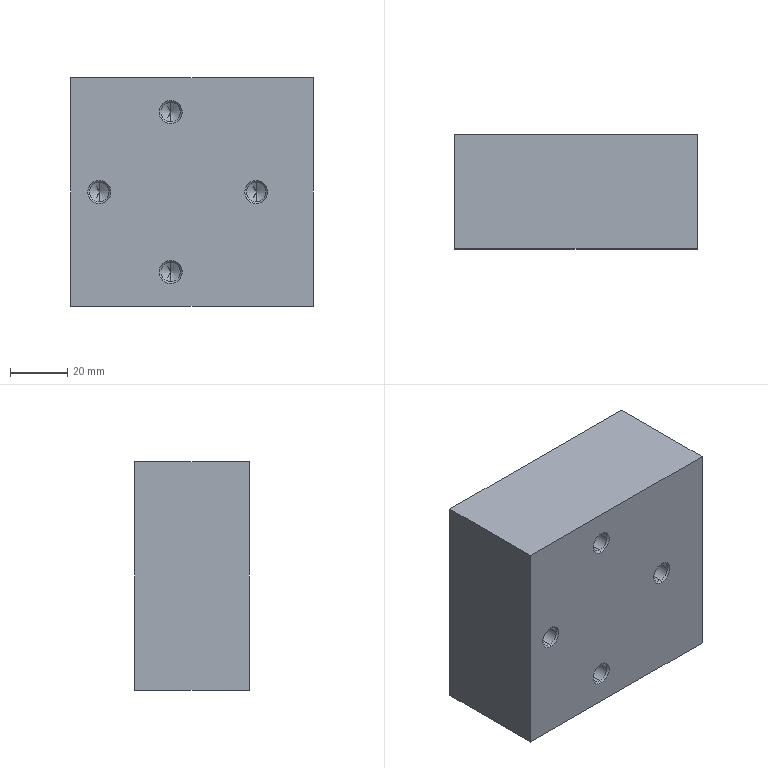Part | SolidWorks | features ICE 2, Extrusion 1, HoleWzd 1 | 1 solid | 45 faces | box 85 x 40 x 80 mm | volume 265399 mm3 | cone 16 | plane 16 | cylinder 13 | commonest cylinder face diameters 6.8 x8 2 x3 16.4 x2
STEP:
#1=CARTESIAN_POINT('',(-7.5,0.625,-24.6));
#2=VERTEX_POINT('',#1);
#3=CARTESIAN_POINT('',(-7.5,0.625,-31.4));
#4=VERTEX_POINT('',#3);
#5=CARTESIAN_POINT('',(-7.5,0.625,-28.));
#6=DIRECTION('',(0.,-1.,0.));
#7=DIRECTION('',(0.,0.,-1.));
#8=AXIS2_PLACEMENT_3D('',#5,#6,#7);
#9=CIRCLE('',#8,3.4);
#10=EDGE_CURVE('',#2,#4,#9,.T.);
#11=ORIENTED_EDGE('',*,*,#10,.F.);
#12=CARTESIAN_POINT('',(-7.5,0.,-23.975));
#13=VERTEX_POINT('',#12);
#14=CARTESIAN_POINT('',(-7.5,0.,-23.975));
#15=DIRECTION('',(0.,-0.7071,0.7071));
#16=VECTOR('',#15,1000.);
#17=LINE('',#14,#16);
#18=EDGE_CURVE('',#2,#13,#17,.T.);
#19=ORIENTED_EDGE('',*,*,#18,.T.);
#20=CARTESIAN_POINT('',(-7.5,0.,-32.025));
#21=VERTEX_POINT('',#20);
#22=CARTESIAN_POINT('',(-7.5,0.,-28.));
#23=DIRECTION('',(0.,-1.,0.));
#24=DIRECTION('',(0.,0.,-1.));
#25=AXIS2_PLACEMENT_3D('',#22,#23,#24);
#26=CIRCLE('',#25,4.025);
#27=EDGE_CURVE('',#13,#21,#26,.T.);
#28=ORIENTED_EDGE('',*,*,#27,.T.);
#29=CARTESIAN_POINT('',(-7.5,0.,-32.025));
#30=DIRECTION('',(0.,-0.7071,-0.7071));
#31=VECTOR('',#30,1000.);
#32=LINE('',#29,#31);
#33=EDGE_CURVE('',#4,#21,#32,.T.);
#34=ORIENTED_EDGE('',*,*,#33,.F.);
#35=EDGE_LOOP('',(#11,#19,#28,#34));
#36=FACE_OUTER_BOUND('',#35,.T.);
#37=CARTESIAN_POINT('',(-7.5,0.,-28.));
#38=DIRECTION('',(0.,-1.,0.));
#39=DIRECTION('',(0.,0.,-1.));
#40=AXIS2_PLACEMENT_3D('',#37,#38,#39);
#41=CONICAL_SURFACE('',#40,4.025,0.7854);
#42=ADVANCED_FACE('',(#36),#41,.F.);
#43=CARTESIAN_POINT('',(-7.5,22.25,-24.6));
#44=VERTEX_POINT('',#43);
#45=CARTESIAN_POINT('',(-7.5,22.25,-31.4));
#46=VERTEX_POINT('',#45);
#47=CARTESIAN_POINT('',(-7.5,22.25,-28.));
#48=DIRECTION('',(0.,-1.,0.));
#49=DIRECTION('',(0.,0.,-1.));
#50=AXIS2_PLACEMENT_3D('',#47,#48,#49);
#51=CIRCLE('',#50,3.4);
#52=EDGE_CURVE('',#44,#46,#51,.T.);
#53=ORIENTED_EDGE('',*,*,#52,.F.);
#54=CARTESIAN_POINT('',(-7.5,0.,-24.6));
#55=DIRECTION('',(0.,-1.,0.));
#56=VECTOR('',#55,1000.);
#57=LINE('',#54,#56);
#58=EDGE_CURVE('',#44,#2,#57,.T.);
#59=ORIENTED_EDGE('',*,*,#58,.T.);
#60=ORIENTED_EDGE('',*,*,#10,.T.);
#61=CARTESIAN_POINT('',(-7.5,0.,-31.4));
#62=DIRECTION('',(0.,-1.,0.));
#63=VECTOR('',#62,1000.);
#64=LINE('',#61,#63);
#65=EDGE_CURVE('',#46,#4,#64,.T.);
#66=ORIENTED_EDGE('',*,*,#65,.F.);
#67=EDGE_LOOP('',(#53,#59,#60,#66));
#68=FACE_OUTER_BOUND('',#67,.T.);
#69=CARTESIAN_POINT('',(-7.5,0.,-28.));
#70=DIRECTION('',(0.,-1.,0.));
#71=DIRECTION('',(0.,0.,-1.));
#72=AXIS2_PLACEMENT_3D('',#69,#70,#71);
#73=CYLINDRICAL_SURFACE('',#72,3.4);
#74=ADVANCED_FACE('',(#68),#73,.F.);
#75=CARTESIAN_POINT('',(-7.5,24.293,-28.));
#76=VERTEX_POINT('',#75);
#77=CARTESIAN_POINT('',(-7.5,22.25,-31.4));
#78=DIRECTION('',(0.,-0.515,-0.8572));
#79=VECTOR('',#78,1000.);
#80=LINE('',#77,#79);
#81=EDGE_CURVE('',#76,#46,#80,.T.);
#82=ORIENTED_EDGE('',*,*,#81,.F.);
#83=CARTESIAN_POINT('',(-7.5,22.25,-24.6));
#84=DIRECTION('',(0.,-0.515,0.8572));
#85=VECTOR('',#84,1000.);
#86=LINE('',#83,#85);
#87=EDGE_CURVE('',#76,#44,#86,.T.);
#88=ORIENTED_EDGE('',*,*,#87,.T.);
#89=ORIENTED_EDGE('',*,*,#52,.T.);
#90=EDGE_LOOP('',(#82,#88,#89));
#91=FACE_OUTER_BOUND('',#90,.T.);
#92=CARTESIAN_POINT('',(-7.5,22.25,-28.));
#93=DIRECTION('',(0.,-1.,0.));
#94=DIRECTION('',(0.,0.,-1.));
#95=AXIS2_PLACEMENT_3D('',#92,#93,#94);
#96=CONICAL_SURFACE('',#95,3.4,1.03);
#97=ADVANCED_FACE('',(#91),#96,.F.);
#98=CARTESIAN_POINT('',(22.5,0.625,3.4));
#99=VERTEX_POINT('',#98);
#100=CARTESIAN_POINT('',(22.5,0.625,-3.4));
#101=VERTEX_POINT('',#100);
#102=CARTESIAN_POINT('',(22.5,0.625,0.));
#103=DIRECTION('',(0.,-1.,0.));
#104=DIRECTION('',(0.,0.,-1.));
#105=AXIS2_PLACEMENT_3D('',#102,#103,#104);
#106=CIRCLE('',#105,3.4);
#107=EDGE_CURVE('',#99,#101,#106,.T.);
#108=ORIENTED_EDGE('',*,*,#107,.F.);
#109=CARTESIAN_POINT('',(22.5,0.,4.025));
#110=VERTEX_POINT('',#109);
#111=CARTESIAN_POINT('',(22.5,0.,4.025));
#112=DIRECTION('',(0.,-0.7071,0.7071));
#113=VECTOR('',#112,1000.);
#114=LINE('',#111,#113);
#115=EDGE_CURVE('',#99,#110,#114,.T.);
#116=ORIENTED_EDGE('',*,*,#115,.T.);
#117=CARTESIAN_POINT('',(22.5,0.,-4.025));
#118=VERTEX_POINT('',#117);
#119=CARTESIAN_POINT('',(22.5,0.,0.));
#120=DIRECTION('',(0.,-1.,0.));
#121=DIRECTION('',(0.,0.,-1.));
#122=AXIS2_PLACEMENT_3D('',#119,#120,#121);
#123=CIRCLE('',#122,4.025);
#124=EDGE_CURVE('',#110,#118,#123,.T.);
#125=ORIENTED_EDGE('',*,*,#124,.T.);
#126=CARTESIAN_POINT('',(22.5,0.,-4.025));
#127=DIRECTION('',(0.,-0.7071,-0.7071));
#128=VECTOR('',#127,1000.);
#129=LINE('',#126,#128);
#130=EDGE_CURVE('',#101,#118,#129,.T.);
#131=ORIENTED_EDGE('',*,*,#130,.F.);
#132=EDGE_LOOP('',(#108,#116,#125,#131));
#133=FACE_OUTER_BOUND('',#132,.T.);
#134=CARTESIAN_POINT('',(22.5,0.,0.));
#135=DIRECTION('',(0.,-1.,0.));
#136=DIRECTION('',(0.,0.,-1.));
#137=AXIS2_PLACEMENT_3D('',#134,#135,#136);
#138=CONICAL_SURFACE('',#137,4.025,0.7854);
#139=ADVANCED_FACE('',(#133),#138,.F.);
#140=CARTESIAN_POINT('',(22.5,22.25,3.4));
#141=VERTEX_POINT('',#140);
#142=CARTESIAN_POINT('',(22.5,22.25,-3.4));
#143=VERTEX_POINT('',#142);
#144=CARTESIAN_POINT('',(22.5,22.25,0.));
#145=DIRECTION('',(0.,-1.,0.));
#146=DIRECTION('',(0.,0.,-1.));
#147=AXIS2_PLACEMENT_3D('',#144,#145,#146);
#148=CIRCLE('',#147,3.4);
#149=EDGE_CURVE('',#141,#143,#148,.T.);
#150=ORIENTED_EDGE('',*,*,#149,.F.);
#151=CARTESIAN_POINT('',(22.5,0.,3.4));
#152=DIRECTION('',(0.,-1.,0.));
#153=VECTOR('',#152,1000.);
#154=LINE('',#151,#153);
#155=EDGE_CURVE('',#141,#99,#154,.T.);
#156=ORIENTED_EDGE('',*,*,#155,.T.);
#157=ORIENTED_EDGE('',*,*,#107,.T.);
#158=CARTESIAN_POINT('',(22.5,0.,-3.4));
#159=DIRECTION('',(0.,-1.,0.));
#160=VECTOR('',#159,1000.);
#161=LINE('',#158,#160);
#162=EDGE_CURVE('',#143,#101,#161,.T.);
#163=ORIENTED_EDGE('',*,*,#162,.F.);
#164=EDGE_LOOP('',(#150,#156,#157,#163));
#165=FACE_OUTER_BOUND('',#164,.T.);
#166=CARTESIAN_POINT('',(22.5,0.,0.));
#167=DIRECTION('',(0.,-1.,0.));
#168=DIRECTION('',(0.,0.,-1.));
#169=AXIS2_PLACEMENT_3D('',#166,#167,#168);
#170=CYLINDRICAL_SURFACE('',#169,3.4);
#171=ADVANCED_FACE('',(#165),#170,.F.);
#172=CARTESIAN_POINT('',(22.5,24.293,0.));
#173=VERTEX_POINT('',#172);
#174=CARTESIAN_POINT('',(22.5,22.25,-3.4));
#175=DIRECTION('',(0.,-0.515,-0.8572));
#176=VECTOR('',#175,1000.);
#177=LINE('',#174,#176);
#178=EDGE_CURVE('',#173,#143,#177,.T.);
#179=ORIENTED_EDGE('',*,*,#178,.F.);
#180=CARTESIAN_POINT('',(22.5,22.25,3.4));
#181=DIRECTION('',(0.,-0.515,0.8572));
#182=VECTOR('',#181,1000.);
#183=LINE('',#180,#182);
#184=EDGE_CURVE('',#173,#141,#183,.T.);
#185=ORIENTED_EDGE('',*,*,#184,.T.);
#186=ORIENTED_EDGE('',*,*,#149,.T.);
#187=EDGE_LOOP('',(#179,#185,#186));
#188=FACE_OUTER_BOUND('',#187,.T.);
#189=CARTESIAN_POINT('',(22.5,22.25,0.));
#190=DIRECTION('',(0.,-1.,0.));
#191=DIRECTION('',(0.,0.,-1.));
#192=AXIS2_PLACEMENT_3D('',#189,#190,#191);
#193=CONICAL_SURFACE('',#192,3.4,1.03);
#194=ADVANCED_FACE('',(#188),#193,.F.);
#195=CARTESIAN_POINT('',(-7.5,0.625,31.4));
#196=VERTEX_POINT('',#195);
#197=CARTESIAN_POINT('',(-7.5,0.625,24.6));
#198=VERTEX_POINT('',#197);
#199=CARTESIAN_POINT('',(-7.5,0.625,28.));
#200=DIRECTION('',(0.,-1.,0.));
#201=DIRECTION('',(0.,0.,-1.));
#202=AXIS2_PLACEMENT_3D('',#199,#200,#201);
#203=CIRCLE('',#202,3.4);
#204=EDGE_CURVE('',#196,#198,#203,.T.);
#205=ORIENTED_EDGE('',*,*,#204,.F.);
#206=CARTESIAN_POINT('',(-7.5,0.,32.025));
#207=VERTEX_POINT('',#206);
#208=CARTESIAN_POINT('',(-7.5,0.,32.025));
#209=DIRECTION('',(0.,-0.7071,0.7071));
#210=VECTOR('',#209,1000.);
#211=LINE('',#208,#210);
#212=EDGE_CURVE('',#196,#207,#211,.T.);
#213=ORIENTED_EDGE('',*,*,#212,.T.);
#214=CARTESIAN_POINT('',(-7.5,0.,23.975));
#215=VERTEX_POINT('',#214);
#216=CARTESIAN_POINT('',(-7.5,0.,28.));
#217=DIRECTION('',(0.,-1.,0.));
#218=DIRECTION('',(0.,0.,-1.));
#219=AXIS2_PLACEMENT_3D('',#216,#217,#218);
#220=CIRCLE('',#219,4.025);
#221=EDGE_CURVE('',#207,#215,#220,.T.);
#222=ORIENTED_EDGE('',*,*,#221,.T.);
#223=CARTESIAN_POINT('',(-7.5,0.,23.975));
#224=DIRECTION('',(0.,-0.7071,-0.7071));
#225=VECTOR('',#224,1000.);
#226=LINE('',#223,#225);
#227=EDGE_CURVE('',#198,#215,#226,.T.);
#228=ORIENTED_EDGE('',*,*,#227,.F.);
#229=EDGE_LOOP('',(#205,#213,#222,#228));
#230=FACE_OUTER_BOUND('',#229,.T.);
#231=CARTESIAN_POINT('',(-7.5,0.,28.));
#232=DIRECTION('',(0.,-1.,0.));
#233=DIRECTION('',(0.,0.,-1.));
#234=AXIS2_PLACEMENT_3D('',#231,#232,#233);
#235=CONICAL_SURFACE('',#234,4.025,0.7854);
#236=ADVANCED_FACE('',(#230),#235,.F.);
#237=CARTESIAN_POINT('',(-7.5,22.25,31.4));
#238=VERTEX_POINT('',#237);
#239=CARTESIAN_POINT('',(-7.5,22.25,24.6));
#240=VERTEX_POINT('',#239);
#241=CARTESIAN_POINT('',(-7.5,22.25,28.));
#242=DIRECTION('',(0.,-1.,0.));
#243=DIRECTION('',(0.,0.,-1.));
#244=AXIS2_PLACEMENT_3D('',#241,#242,#243);
#245=CIRCLE('',#244,3.4);
#246=EDGE_CURVE('',#238,#240,#245,.T.);
#247=ORIENTED_EDGE('',*,*,#246,.F.);
#248=CARTESIAN_POINT('',(-7.5,0.,31.4));
#249=DIRECTION('',(0.,-1.,0.));
#250=VECTOR('',#249,1000.);
#251=LINE('',#248,#250);
#252=EDGE_CURVE('',#238,#196,#251,.T.);
#253=ORIENTED_EDGE('',*,*,#252,.T.);
#254=ORIENTED_EDGE('',*,*,#204,.T.);
#255=CARTESIAN_POINT('',(-7.5,0.,24.6));
#256=DIRECTION('',(0.,-1.,0.));
#257=VECTOR('',#256,1000.);
#258=LINE('',#255,#257);
#259=EDGE_CURVE('',#240,#198,#258,.T.);
#260=ORIENTED_EDGE('',*,*,#259,.F.);
#261=EDGE_LOOP('',(#247,#253,#254,#260));
#262=FACE_OUTER_BOUND('',#261,.T.);
#263=CARTESIAN_POINT('',(-7.5,0.,28.));
#264=DIRECTION('',(0.,-1.,0.));
#265=DIRECTION('',(0.,0.,-1.));
#266=AXIS2_PLACEMENT_3D('',#263,#264,#265);
#267=CYLINDRICAL_SURFACE('',#266,3.4);
#268=ADVANCED_FACE('',(#262),#267,.F.);
#269=CARTESIAN_POINT('',(-7.5,24.293,28.));
#270=VERTEX_POINT('',#269);
#271=CARTESIAN_POINT('',(-7.5,22.25,24.6));
#272=DIRECTION('',(0.,-0.515,-0.8572));
#273=VECTOR('',#272,1000.);
#274=LINE('',#271,#273);
#275=EDGE_CURVE('',#270,#240,#274,.T.);
#276=ORIENTED_EDGE('',*,*,#275,.F.);
#277=CARTESIAN_POINT('',(-7.5,22.25,31.4));
#278=DIRECTION('',(0.,-0.515,0.8572));
#279=VECTOR('',#278,1000.);
#280=LINE('',#277,#279);
#281=EDGE_CURVE('',#270,#238,#280,.T.);
#282=ORIENTED_EDGE('',*,*,#281,.T.);
#283=ORIENTED_EDGE('',*,*,#246,.T.);
#284=EDGE_LOOP('',(#276,#282,#283));
#285=FACE_OUTER_BOUND('',#284,.T.);
#286=CARTESIAN_POINT('',(-7.5,22.25,28.));
#287=DIRECTION('',(0.,-1.,0.));
#288=DIRECTION('',(0.,0.,-1.));
#289=AXIS2_PLACEMENT_3D('',#286,#287,#288);
#290=CONICAL_SURFACE('',#289,3.4,1.03);
#291=ADVANCED_FACE('',(#285),#290,.F.);
#292=CARTESIAN_POINT('',(-32.5,0.625,3.4));
#293=VERTEX_POINT('',#292);
#294=CARTESIAN_POINT('',(-32.5,0.625,-3.4));
#295=VERTEX_POINT('',#294);
#296=CARTESIAN_POINT('',(-32.5,0.625,0.));
#297=DIRECTION('',(0.,-1.,0.));
#298=DIRECTION('',(0.,0.,-1.));
#299=AXIS2_PLACEMENT_3D('',#296,#297,#298);
#300=CIRCLE('',#299,3.4);
#301=EDGE_CURVE('',#293,#295,#300,.T.);
#302=ORIENTED_EDGE('',*,*,#301,.F.);
#303=CARTESIAN_POINT('',(-32.5,0.,4.025));
#304=VERTEX_POINT('',#303);
#305=CARTESIAN_POINT('',(-32.5,0.,4.025));
#306=DIRECTION('',(0.,-0.7071,0.7071));
#307=VECTOR('',#306,1000.);
#308=LINE('',#305,#307);
#309=EDGE_CURVE('',#293,#304,#308,.T.);
#310=ORIENTED_EDGE('',*,*,#309,.T.);
#311=CARTESIAN_POINT('',(-32.5,0.,-4.025));
#312=VERTEX_POINT('',#311);
#313=CARTESIAN_POINT('',(-32.5,0.,0.));
#314=DIRECTION('',(0.,-1.,0.));
#315=DIRECTION('',(0.,0.,-1.));
#316=AXIS2_PLACEMENT_3D('',#313,#314,#315);
#317=CIRCLE('',#316,4.025);
#318=EDGE_CURVE('',#304,#312,#317,.T.);
#319=ORIENTED_EDGE('',*,*,#318,.T.);
#320=CARTESIAN_POINT('',(-32.5,0.,-4.025));
#321=DIRECTION('',(0.,-0.7071,-0.7071));
#322=VECTOR('',#321,1000.);
#323=LINE('',#320,#322);
#324=EDGE_CURVE('',#295,#312,#323,.T.);
#325=ORIENTED_EDGE('',*,*,#324,.F.);
#326=EDGE_LOOP('',(#302,#310,#319,#325));
#327=FACE_OUTER_BOUND('',#326,.T.);
#328=CARTESIAN_POINT('',(-32.5,0.,0.));
#329=DIRECTION('',(0.,-1.,0.));
#330=DIRECTION('',(0.,0.,-1.));
#331=AXIS2_PLACEMENT_3D('',#328,#329,#330);
#332=CONICAL_SURFACE('',#331,4.025,0.7854);
#333=ADVANCED_FACE('',(#327),#332,.F.);
#334=CARTESIAN_POINT('',(-32.5,22.25,3.4));
#335=VERTEX_POINT('',#334);
#336=CARTESIAN_POINT('',(-32.5,22.25,-3.4));
#337=VERTEX_POINT('',#336);
#338=CARTESIAN_POINT('',(-32.5,22.25,0.));
#339=DIRECTION('',(0.,-1.,0.));
#340=DIRECTION('',(0.,0.,-1.));
#341=AXIS2_PLACEMENT_3D('',#338,#339,#340);
#342=CIRCLE('',#341,3.4);
#343=EDGE_CURVE('',#335,#337,#342,.T.);
#344=ORIENTED_EDGE('',*,*,#343,.F.);
#345=CARTESIAN_POINT('',(-32.5,0.,3.4));
#346=DIRECTION('',(0.,-1.,0.));
#347=VECTOR('',#346,1000.);
#348=LINE('',#345,#347);
#349=EDGE_CURVE('',#335,#293,#348,.T.);
#350=ORIENTED_EDGE('',*,*,#349,.T.);
#351=ORIENTED_EDGE('',*,*,#301,.T.);
#352=CARTESIAN_POINT('',(-32.5,0.,-3.4));
#353=DIRECTION('',(0.,-1.,0.));
#354=VECTOR('',#353,1000.);
#355=LINE('',#352,#354);
#356=EDGE_CURVE('',#337,#295,#355,.T.);
#357=ORIENTED_EDGE('',*,*,#356,.F.);
#358=EDGE_LOOP('',(#344,#350,#351,#357));
#359=FACE_OUTER_BOUND('',#358,.T.);
#360=CARTESIAN_POINT('',(-32.5,0.,0.));
#361=DIRECTION('',(0.,-1.,0.));
#362=DIRECTION('',(0.,0.,-1.));
#363=AXIS2_PLACEMENT_3D('',#360,#361,#362);
#364=CYLINDRICAL_SURFACE('',#363,3.4);
#365=ADVANCED_FACE('',(#359),#364,.F.);
#366=CARTESIAN_POINT('',(-32.5,24.293,0.));
#367=VERTEX_POINT('',#366);
#368=CARTESIAN_POINT('',(-32.5,22.25,-3.4));
#369=DIRECTION('',(0.,-0.515,-0.8572));
#370=VECTOR('',#369,1000.);
#371=LINE('',#368,#370);
#372=EDGE_CURVE('',#367,#337,#371,.T.);
#373=ORIENTED_EDGE('',*,*,#372,.F.);
#374=CARTESIAN_POINT('',(-32.5,22.25,3.4));
#375=DIRECTION('',(0.,-0.515,0.8572));
#376=VECTOR('',#375,1000.);
#377=LINE('',#374,#376);
#378=EDGE_CURVE('',#367,#335,#377,.T.);
#379=ORIENTED_EDGE('',*,*,#378,.T.);
#380=ORIENTED_EDGE('',*,*,#343,.T.);
#381=EDGE_LOOP('',(#373,#379,#380));
#382=FACE_OUTER_BOUND('',#381,.T.);
#383=CARTESIAN_POINT('',(-32.5,22.25,0.));
#384=DIRECTION('',(0.,-1.,0.));
#385=DIRECTION('',(0.,0.,-1.));
#386=AXIS2_PLACEMENT_3D('',#383,#384,#385);
#387=CONICAL_SURFACE('',#386,3.4,1.03);
#388=ADVANCED_FACE('',(#382),#387,.F.);
#389=CARTESIAN_POINT('',(2.5,39.,-8.139));
#390=VERTEX_POINT('',#389);
#391=CARTESIAN_POINT('',(2.5,39.,-27.15));
#392=VERTEX_POINT('',#391);
#393=CARTESIAN_POINT('',(2.5,39.,-27.15));
#394=DIRECTION('',(0.,0.,-1.));
#395=VECTOR('',#394,1000.);
#396=LINE('',#393,#395);
#397=EDGE_CURVE('',#390,#392,#396,.T.);
#398=ORIENTED_EDGE('',*,*,#397,.F.);
#399=CARTESIAN_POINT('',(2.5,40.,-8.2));
#400=VERTEX_POINT('',#399);
#401=CARTESIAN_POINT('',(2.5,40.,0.));
#402=DIRECTION('',(1.,0.,0.));
#403=DIRECTION('',(0.,0.,-1.));
#404=AXIS2_PLACEMENT_3D('',#401,#402,#403);
#405=CIRCLE('',#404,8.2);
#406=EDGE_CURVE('',#390,#400,#405,.T.);
#407=ORIENTED_EDGE('',*,*,#406,.T.);
#408=CARTESIAN_POINT('',(2.5,40.,-27.15));
#409=VERTEX_POINT('',#408);
#410=CARTESIAN_POINT('',(2.5,40.,-27.15));
#411=DIRECTION('',(0.,0.,-1.));
#412=VECTOR('',#411,1000.);
#413=LINE('',#410,#412);
#414=EDGE_CURVE('',#400,#409,#413,.T.);
#415=ORIENTED_EDGE('',*,*,#414,.T.);
#416=CARTESIAN_POINT('',(2.5,39.,-27.15));
#417=DIRECTION('',(0.,1.,0.));
#418=VECTOR('',#417,1000.);
#419=LINE('',#416,#418);
#420=EDGE_CURVE('',#392,#409,#419,.T.);
#421=ORIENTED_EDGE('',*,*,#420,.F.);
#422=EDGE_LOOP('',(#398,#407,#415,#421));
#423=FACE_OUTER_BOUND('',#422,.T.);
#424=CARTESIAN_POINT('',(2.5,39.,-27.15));
#425=DIRECTION('',(1.,0.,0.));
#426=DIRECTION('',(0.,0.,-1.));
#427=AXIS2_PLACEMENT_3D('',#424,#425,#426);
#428=PLANE('',#427);
#429=ADVANCED_FACE('',(#423),#428,.F.);
#430=CARTESIAN_POINT('',(-17.5,40.,-27.15));
#431=VERTEX_POINT('',#430);
#432=CARTESIAN_POINT('',(-17.5,40.,-8.2));
#433=VERTEX_POINT('',#432);
#434=CARTESIAN_POINT('',(-17.5,40.,-27.15));
#435=DIRECTION('',(0.,0.,1.));
#436=VECTOR('',#435,1000.);
#437=LINE('',#434,#436);
#438=EDGE_CURVE('',#431,#433,#437,.T.);
#439=ORIENTED_EDGE('',*,*,#438,.T.);
#440=CARTESIAN_POINT('',(-17.5,39.,-8.139));
#441=VERTEX_POINT('',#440);
#442=CARTESIAN_POINT('',(-17.5,40.,0.));
#443=DIRECTION('',(-1.,0.,0.));
#444=DIRECTION('',(0.,0.,1.));
#445=AXIS2_PLACEMENT_3D('',#442,#443,#444);
#446=CIRCLE('',#445,8.2);
#447=EDGE_CURVE('',#433,#441,#446,.T.);
#448=ORIENTED_EDGE('',*,*,#447,.T.);
#449=CARTESIAN_POINT('',(-17.5,39.,-27.15));
#450=VERTEX_POINT('',#449);
#451=CARTESIAN_POINT('',(-17.5,39.,-27.15));
#452=DIRECTION('',(0.,0.,1.));
#453=VECTOR('',#452,1000.);
#454=LINE('',#451,#453);
#455=EDGE_CURVE('',#450,#441,#454,.T.);
#456=ORIENTED_EDGE('',*,*,#455,.F.);
#457=CARTESIAN_POINT('',(-17.5,39.,-27.15));
#458=DIRECTION('',(0.,1.,0.));
#459=VECTOR('',#458,1000.);
#460=LINE('',#457,#459);
#461=EDGE_CURVE('',#450,#431,#460,.T.);
#462=ORIENTED_EDGE('',*,*,#461,.T.);
#463=EDGE_LOOP('',(#439,#448,#456,#462));
#464=FACE_OUTER_BOUND('',#463,.T.);
#465=CARTESIAN_POINT('',(-17.5,39.,-27.15));
#466=DIRECTION('',(-1.,0.,0.));
#467=DIRECTION('',(0.,0.,1.));
#468=AXIS2_PLACEMENT_3D('',#465,#466,#467);
#469=PLANE('',#468);
#470=ADVANCED_FACE('',(#464),#469,.F.);
#471=CARTESIAN_POINT('',(4.5,39.,-8.139));
#472=DIRECTION('',(-1.,0.,0.));
#473=VECTOR('',#472,1000.);
#474=LINE('',#471,#473);
#475=EDGE_CURVE('',#390,#441,#474,.T.);
#476=ORIENTED_EDGE('',*,*,#475,.F.);
#477=ORIENTED_EDGE('',*,*,#397,.T.);
#478=CARTESIAN_POINT('',(-17.5,39.,-27.15));
#479=DIRECTION('',(-1.,0.,0.));
#480=VECTOR('',#479,1000.);
#481=LINE('',#478,#480);
#482=EDGE_CURVE('',#392,#450,#481,.T.);
#483=ORIENTED_EDGE('',*,*,#482,.T.);
#484=ORIENTED_EDGE('',*,*,#455,.T.);
#485=EDGE_LOOP('',(#476,#477,#483,#484));
#486=FACE_OUTER_BOUND('',#485,.T.);
#487=CARTESIAN_POINT('',(0.,39.,0.));
#488=DIRECTION('',(0.,1.,0.));
#489=DIRECTION('',(0.,0.,1.));
#490=AXIS2_PLACEMENT_3D('',#487,#488,#489);
#491=PLANE('',#490);
#492=ADVANCED_FACE('',(#486),#491,.T.);
#493=CARTESIAN_POINT('',(42.5,0.,40.));
#494=VERTEX_POINT('',#493);
#495=CARTESIAN_POINT('',(42.5,0.,-40.));
#496=VERTEX_POINT('',#495);
#497=CARTESIAN_POINT('',(42.5,0.,40.));
#498=DIRECTION('',(0.,0.,-1.));
#499=VECTOR('',#498,1000.);
#500=LINE('',#497,#499);
#501=EDGE_CURVE('',#494,#496,#500,.T.);
#502=ORIENTED_EDGE('',*,*,#501,.T.);
#503=CARTESIAN_POINT('',(42.5,40.,-40.));
#504=VERTEX_POINT('',#503);
#505=CARTESIAN_POINT('',(42.5,40.,-40.));
#506=DIRECTION('',(0.,-1.,0.));
#507=VECTOR('',#506,1000.);
#508=LINE('',#505,#507);
#509=EDGE_CURVE('',#504,#496,#508,.T.);
#510=ORIENTED_EDGE('',*,*,#509,.F.);
#511=CARTESIAN_POINT('',(42.5,40.,40.));
#512=VERTEX_POINT('',#511);
#513=CARTESIAN_POINT('',(42.5,40.,40.));
#514=DIRECTION('',(0.,0.,-1.));
#515=VECTOR('',#514,1000.);
#516=LINE('',#513,#515);
#517=EDGE_CURVE('',#512,#504,#516,.T.);
#518=ORIENTED_EDGE('',*,*,#517,.F.);
#519=CARTESIAN_POINT('',(42.5,40.,40.));
#520=DIRECTION('',(0.,-1.,0.));
#521=VECTOR('',#520,1000.);
#522=LINE('',#519,#521);
#523=EDGE_CURVE('',#512,#494,#522,.T.);
#524=ORIENTED_EDGE('',*,*,#523,.T.);
#525=EDGE_LOOP('',(#502,#510,#518,#524));
#526=FACE_OUTER_BOUND('',#525,.T.);
#527=CARTESIAN_POINT('',(42.5,40.,40.));
#528=DIRECTION('',(-1.,0.,0.));
#529=DIRECTION('',(0.,0.,1.));
#530=AXIS2_PLACEMENT_3D('',#527,#528,#529);
#531=PLANE('',#530);
#532=ADVANCED_FACE('',(#526),#531,.F.);
#533=CARTESIAN_POINT('',(-42.5,0.,-40.));
#534=VERTEX_POINT('',#533);
#535=CARTESIAN_POINT('',(-42.5,0.,-40.));
#536=DIRECTION('',(-1.,0.,0.));
#537=VECTOR('',#536,1000.);
#538=LINE('',#535,#537);
#539=EDGE_CURVE('',#496,#534,#538,.T.);
#540=ORIENTED_EDGE('',*,*,#539,.T.);
#541=CARTESIAN_POINT('',(-42.5,40.,-40.));
#542=VERTEX_POINT('',#541);
#543=CARTESIAN_POINT('',(-42.5,40.,-40.));
#544=DIRECTION('',(0.,-1.,0.));
#545=VECTOR('',#544,1000.);
#546=LINE('',#543,#545);
#547=EDGE_CURVE('',#542,#534,#546,.T.);
#548=ORIENTED_EDGE('',*,*,#547,.F.);
#549=CARTESIAN_POINT('',(-42.5,40.,-40.));
#550=DIRECTION('',(-1.,0.,0.));
#551=VECTOR('',#550,1000.);
#552=LINE('',#549,#551);
#553=EDGE_CURVE('',#504,#542,#552,.T.);
#554=ORIENTED_EDGE('',*,*,#553,.F.);
#555=ORIENTED_EDGE('',*,*,#509,.T.);
#556=EDGE_LOOP('',(#540,#548,#554,#555));
#557=FACE_OUTER_BOUND('',#556,.T.);
#558=CARTESIAN_POINT('',(-42.5,40.,-40.));
#559=DIRECTION('',(0.,0.,1.));
#560=DIRECTION('',(1.,0.,0.));
#561=AXIS2_PLACEMENT_3D('',#558,#559,#560);
#562=PLANE('',#561);
#563=ADVANCED_FACE('',(#557),#562,.F.);
#564=CARTESIAN_POINT('',(-42.5,0.,40.));
#565=VERTEX_POINT('',#564);
#566=CARTESIAN_POINT('',(-42.5,0.,40.));
#567=DIRECTION('',(0.,0.,1.));
#568=VECTOR('',#567,1000.);
#569=LINE('',#566,#568);
#570=EDGE_CURVE('',#534,#565,#569,.T.);
#571=ORIENTED_EDGE('',*,*,#570,.T.);
#572=CARTESIAN_POINT('',(-42.5,40.,40.));
#573=VERTEX_POINT('',#572);
#574=CARTESIAN_POINT('',(-42.5,40.,40.));
#575=DIRECTION('',(0.,-1.,0.));
#576=VECTOR('',#575,1000.);
#577=LINE('',#574,#576);
#578=EDGE_CURVE('',#573,#565,#577,.T.);
#579=ORIENTED_EDGE('',*,*,#578,.F.);
#580=CARTESIAN_POINT('',(-42.5,40.,40.));
#581=DIRECTION('',(0.,0.,1.));
#582=VECTOR('',#581,1000.);
#583=LINE('',#580,#582);
#584=EDGE_CURVE('',#542,#573,#583,.T.);
#585=ORIENTED_EDGE('',*,*,#584,.F.);
#586=ORIENTED_EDGE('',*,*,#547,.T.);
#587=EDGE_LOOP('',(#571,#579,#585,#586));
#588=FACE_OUTER_BOUND('',#587,.T.);
#589=CARTESIAN_POINT('',(-42.5,40.,40.));
#590=DIRECTION('',(1.,0.,0.));
#591=DIRECTION('',(0.,0.,-1.));
#592=AXIS2_PLACEMENT_3D('',#589,#590,#591);
#593=PLANE('',#592);
#594=ADVANCED_FACE('',(#588),#593,.F.);
#595=CARTESIAN_POINT('',(-42.5,0.,40.));
#596=DIRECTION('',(1.,0.,0.));
#597=VECTOR('',#596,1000.);
#598=LINE('',#595,#597);
#599=EDGE_CURVE('',#565,#494,#598,.T.);
#600=ORIENTED_EDGE('',*,*,#599,.T.);
#601=ORIENTED_EDGE('',*,*,#523,.F.);
#602=CARTESIAN_POINT('',(-42.5,40.,40.));
#603=DIRECTION('',(1.,0.,0.));
#604=VECTOR('',#603,1000.);
#605=LINE('',#602,#604);
#606=EDGE_CURVE('',#573,#512,#605,.T.);
#607=ORIENTED_EDGE('',*,*,#606,.F.);
#608=ORIENTED_EDGE('',*,*,#578,.T.);
#609=EDGE_LOOP('',(#600,#601,#607,#608));
#610=FACE_OUTER_BOUND('',#609,.T.);
#611=CARTESIAN_POINT('',(-42.5,40.,40.));
#612=DIRECTION('',(0.,0.,-1.));
#613=DIRECTION('',(-1.,0.,0.));
#614=AXIS2_PLACEMENT_3D('',#611,#612,#613);
#615=PLANE('',#614);
#616=ADVANCED_FACE('',(#610),#615,.F.);
#617=ORIENTED_EDGE('',*,*,#414,.F.);
#618=CARTESIAN_POINT('',(4.5,40.,-8.2));
#619=VERTEX_POINT('',#618);
#620=CARTESIAN_POINT('',(4.5,40.,-8.2));
#621=DIRECTION('',(-1.,0.,0.));
#622=VECTOR('',#621,1000.);
#623=LINE('',#620,#622);
#624=EDGE_CURVE('',#619,#400,#623,.T.);
#625=ORIENTED_EDGE('',*,*,#624,.F.);
#626=CARTESIAN_POINT('',(4.5,40.,8.2));
#627=VERTEX_POINT('',#626);
#628=CARTESIAN_POINT('',(4.5,40.,-8.2));
#629=DIRECTION('',(0.,0.,-1.));
#630=VECTOR('',#629,1000.);
#631=LINE('',#628,#630);
#632=EDGE_CURVE('',#627,#619,#631,.T.);
#633=ORIENTED_EDGE('',*,*,#632,.F.);
#634=CARTESIAN_POINT('',(2.5,40.,8.2));
#635=VERTEX_POINT('',#634);
#636=CARTESIAN_POINT('',(4.5,40.,8.2));
#637=DIRECTION('',(-1.,0.,0.));
#638=VECTOR('',#637,1000.);
#639=LINE('',#636,#638);
#640=EDGE_CURVE('',#627,#635,#639,.T.);
#641=ORIENTED_EDGE('',*,*,#640,.T.);
#642=CARTESIAN_POINT('',(2.5,40.,27.15));
#643=VERTEX_POINT('',#642);
#644=CARTESIAN_POINT('',(2.5,40.,-27.15));
#645=DIRECTION('',(0.,0.,-1.));
#646=VECTOR('',#645,1000.);
#647=LINE('',#644,#646);
#648=EDGE_CURVE('',#643,#635,#647,.T.);
#649=ORIENTED_EDGE('',*,*,#648,.F.);
#650=CARTESIAN_POINT('',(-17.5,40.,27.15));
#651=VERTEX_POINT('',#650);
#652=CARTESIAN_POINT('',(-17.5,40.,27.15));
#653=DIRECTION('',(1.,0.,0.));
#654=VECTOR('',#653,1000.);
#655=LINE('',#652,#654);
#656=EDGE_CURVE('',#651,#643,#655,.T.);
#657=ORIENTED_EDGE('',*,*,#656,.F.);
#658=CARTESIAN_POINT('',(-17.5,40.,8.2));
#659=VERTEX_POINT('',#658);
#660=CARTESIAN_POINT('',(-17.5,40.,-27.15));
#661=DIRECTION('',(0.,0.,1.));
#662=VECTOR('',#661,1000.);
#663=LINE('',#660,#662);
#664=EDGE_CURVE('',#659,#651,#663,.T.);
#665=ORIENTED_EDGE('',*,*,#664,.F.);
#666=CARTESIAN_POINT('',(-19.5,40.,8.2));
#667=VERTEX_POINT('',#666);
#668=CARTESIAN_POINT('',(4.5,40.,8.2));
#669=DIRECTION('',(-1.,0.,0.));
#670=VECTOR('',#669,1000.);
#671=LINE('',#668,#670);
#672=EDGE_CURVE('',#659,#667,#671,.T.);
#673=ORIENTED_EDGE('',*,*,#672,.T.);
#674=CARTESIAN_POINT('',(-19.5,40.,-8.2));
#675=VERTEX_POINT('',#674);
#676=CARTESIAN_POINT('',(-19.5,40.,-8.2));
#677=DIRECTION('',(0.,0.,-1.));
#678=VECTOR('',#677,1000.);
#679=LINE('',#676,#678);
#680=EDGE_CURVE('',#667,#675,#679,.T.);
#681=ORIENTED_EDGE('',*,*,#680,.T.);
#682=CARTESIAN_POINT('',(4.5,40.,-8.2));
#683=DIRECTION('',(-1.,0.,0.));
#684=VECTOR('',#683,1000.);
#685=LINE('',#682,#684);
#686=EDGE_CURVE('',#433,#675,#685,.T.);
#687=ORIENTED_EDGE('',*,*,#686,.F.);
#688=ORIENTED_EDGE('',*,*,#438,.F.);
#689=CARTESIAN_POINT('',(-17.5,40.,-27.15));
#690=DIRECTION('',(-1.,0.,0.));
#691=VECTOR('',#690,1000.);
#692=LINE('',#689,#691);
#693=EDGE_CURVE('',#409,#431,#692,.T.);
#694=ORIENTED_EDGE('',*,*,#693,.F.);
#695=EDGE_LOOP('',(#617,#625,#633,#641,#649,#657,#665,#673,#681,#687,#688,#694));
#696=FACE_BOUND('',#695,.T.);
#697=ORIENTED_EDGE('',*,*,#517,.T.);
#698=ORIENTED_EDGE('',*,*,#553,.T.);
#699=ORIENTED_EDGE('',*,*,#584,.T.);
#700=ORIENTED_EDGE('',*,*,#606,.T.);
#701=EDGE_LOOP('',(#697,#698,#699,#700));
#702=FACE_OUTER_BOUND('',#701,.T.);
#703=CARTESIAN_POINT('',(0.,40.,0.));
#704=DIRECTION('',(0.,-1.,0.));
#705=DIRECTION('',(0.,0.,-1.));
#706=AXIS2_PLACEMENT_3D('',#703,#704,#705);
#707=PLANE('',#706);
#708=ADVANCED_FACE('',(#696,#702),#707,.F.);
#709=CARTESIAN_POINT('',(-7.5,0.,-28.));
#710=DIRECTION('',(0.,-1.,0.));
#711=DIRECTION('',(0.,0.,-1.));
#712=AXIS2_PLACEMENT_3D('',#709,#710,#711);
#713=CIRCLE('',#712,4.025);
#714=EDGE_CURVE('',#21,#13,#713,.T.);
#715=ORIENTED_EDGE('',*,*,#714,.F.);
#716=ORIENTED_EDGE('',*,*,#27,.F.);
#717=EDGE_LOOP('',(#715,#716));
#718=FACE_BOUND('',#717,.T.);
#719=CARTESIAN_POINT('',(22.5,0.,0.));
#720=DIRECTION('',(0.,-1.,0.));
#721=DIRECTION('',(0.,0.,-1.));
#722=AXIS2_PLACEMENT_3D('',#719,#720,#721);
#723=CIRCLE('',#722,4.025);
#724=EDGE_CURVE('',#118,#110,#723,.T.);
#725=ORIENTED_EDGE('',*,*,#724,.F.);
#726=ORIENTED_EDGE('',*,*,#124,.F.);
#727=EDGE_LOOP('',(#725,#726));
#728=FACE_BOUND('',#727,.T.);
#729=CARTESIAN_POINT('',(-7.5,0.,28.));
#730=DIRECTION('',(0.,-1.,0.));
#731=DIRECTION('',(0.,0.,-1.));
#732=AXIS2_PLACEMENT_3D('',#729,#730,#731);
#733=CIRCLE('',#732,4.025);
#734=EDGE_CURVE('',#215,#207,#733,.T.);
#735=ORIENTED_EDGE('',*,*,#734,.F.);
#736=ORIENTED_EDGE('',*,*,#221,.F.);
#737=EDGE_LOOP('',(#735,#736));
#738=FACE_BOUND('',#737,.T.);
#739=CARTESIAN_POINT('',(-32.5,0.,0.));
#740=DIRECTION('',(0.,-1.,0.));
#741=DIRECTION('',(0.,0.,-1.));
#742=AXIS2_PLACEMENT_3D('',#739,#740,#741);
#743=CIRCLE('',#742,4.025);
#744=EDGE_CURVE('',#312,#304,#743,.T.);
#745=ORIENTED_EDGE('',*,*,#744,.F.);
#746=ORIENTED_EDGE('',*,*,#318,.F.);
#747=EDGE_LOOP('',(#745,#746));
#748=FACE_BOUND('',#747,.T.);
#749=ORIENTED_EDGE('',*,*,#501,.F.);
#750=ORIENTED_EDGE('',*,*,#599,.F.);
#751=ORIENTED_EDGE('',*,*,#570,.F.);
#752=ORIENTED_EDGE('',*,*,#539,.F.);
#753=EDGE_LOOP('',(#749,#750,#751,#752));
#754=FACE_OUTER_BOUND('',#753,.T.);
#755=CARTESIAN_POINT('',(0.,0.,0.));
#756=DIRECTION('',(0.,-1.,0.));
#757=DIRECTION('',(0.,0.,-1.));
#758=AXIS2_PLACEMENT_3D('',#755,#756,#757);
#759=PLANE('',#758);
#760=ADVANCED_FACE('',(#718,#728,#738,#748,#754),#759,.T.);
#761=ORIENTED_EDGE('',*,*,#378,.F.);
#762=ORIENTED_EDGE('',*,*,#372,.T.);
#763=CARTESIAN_POINT('',(-32.5,22.25,0.));
#764=DIRECTION('',(0.,-1.,0.));
#765=DIRECTION('',(0.,0.,-1.));
#766=AXIS2_PLACEMENT_3D('',#763,#764,#765);
#767=CIRCLE('',#766,3.4);
#768=EDGE_CURVE('',#337,#335,#767,.T.);
#769=ORIENTED_EDGE('',*,*,#768,.T.);
#770=EDGE_LOOP('',(#761,#762,#769));
#771=FACE_OUTER_BOUND('',#770,.T.);
#772=CARTESIAN_POINT('',(-32.5,22.25,0.));
#773=DIRECTION('',(0.,-1.,0.));
#774=DIRECTION('',(0.,0.,-1.));
#775=AXIS2_PLACEMENT_3D('',#772,#773,#774);
#776=CONICAL_SURFACE('',#775,3.4,1.03);
#777=ADVANCED_FACE('',(#771),#776,.F.);
#778=ORIENTED_EDGE('',*,*,#349,.F.);
#779=ORIENTED_EDGE('',*,*,#768,.F.);
#780=ORIENTED_EDGE('',*,*,#356,.T.);
#781=CARTESIAN_POINT('',(-32.5,0.625,0.));
#782=DIRECTION('',(0.,-1.,0.));
#783=DIRECTION('',(0.,0.,-1.));
#784=AXIS2_PLACEMENT_3D('',#781,#782,#783);
#785=CIRCLE('',#784,3.4);
#786=EDGE_CURVE('',#295,#293,#785,.T.);
#787=ORIENTED_EDGE('',*,*,#786,.T.);
#788=EDGE_LOOP('',(#778,#779,#780,#787));
#789=FACE_OUTER_BOUND('',#788,.T.);
#790=CARTESIAN_POINT('',(-32.5,0.,0.));
#791=DIRECTION('',(0.,-1.,0.));
#792=DIRECTION('',(0.,0.,-1.));
#793=AXIS2_PLACEMENT_3D('',#790,#791,#792);
#794=CYLINDRICAL_SURFACE('',#793,3.4);
#795=ADVANCED_FACE('',(#789),#794,.F.);
#796=ORIENTED_EDGE('',*,*,#309,.F.);
#797=ORIENTED_EDGE('',*,*,#786,.F.);
#798=ORIENTED_EDGE('',*,*,#324,.T.);
#799=ORIENTED_EDGE('',*,*,#744,.T.);
#800=EDGE_LOOP('',(#796,#797,#798,#799));
#801=FACE_OUTER_BOUND('',#800,.T.);
#802=CARTESIAN_POINT('',(-32.5,0.,0.));
#803=DIRECTION('',(0.,-1.,0.));
#804=DIRECTION('',(0.,0.,-1.));
#805=AXIS2_PLACEMENT_3D('',#802,#803,#804);
#806=CONICAL_SURFACE('',#805,4.025,0.7854);
#807=ADVANCED_FACE('',(#801),#806,.F.);
#808=ORIENTED_EDGE('',*,*,#281,.F.);
#809=ORIENTED_EDGE('',*,*,#275,.T.);
#810=CARTESIAN_POINT('',(-7.5,22.25,28.));
#811=DIRECTION('',(0.,-1.,0.));
#812=DIRECTION('',(0.,0.,-1.));
#813=AXIS2_PLACEMENT_3D('',#810,#811,#812);
#814=CIRCLE('',#813,3.4);
#815=EDGE_CURVE('',#240,#238,#814,.T.);
#816=ORIENTED_EDGE('',*,*,#815,.T.);
#817=EDGE_LOOP('',(#808,#809,#816));
#818=FACE_OUTER_BOUND('',#817,.T.);
#819=CARTESIAN_POINT('',(-7.5,22.25,28.));
#820=DIRECTION('',(0.,-1.,0.));
#821=DIRECTION('',(0.,0.,-1.));
#822=AXIS2_PLACEMENT_3D('',#819,#820,#821);
#823=CONICAL_SURFACE('',#822,3.4,1.03);
#824=ADVANCED_FACE('',(#818),#823,.F.);
#825=ORIENTED_EDGE('',*,*,#252,.F.);
#826=ORIENTED_EDGE('',*,*,#815,.F.);
#827=ORIENTED_EDGE('',*,*,#259,.T.);
#828=CARTESIAN_POINT('',(-7.5,0.625,28.));
#829=DIRECTION('',(0.,-1.,0.));
#830=DIRECTION('',(0.,0.,-1.));
#831=AXIS2_PLACEMENT_3D('',#828,#829,#830);
#832=CIRCLE('',#831,3.4);
#833=EDGE_CURVE('',#198,#196,#832,.T.);
#834=ORIENTED_EDGE('',*,*,#833,.T.);
#835=EDGE_LOOP('',(#825,#826,#827,#834));
#836=FACE_OUTER_BOUND('',#835,.T.);
#837=CARTESIAN_POINT('',(-7.5,0.,28.));
#838=DIRECTION('',(0.,-1.,0.));
#839=DIRECTION('',(0.,0.,-1.));
#840=AXIS2_PLACEMENT_3D('',#837,#838,#839);
#841=CYLINDRICAL_SURFACE('',#840,3.4);
#842=ADVANCED_FACE('',(#836),#841,.F.);
#843=ORIENTED_EDGE('',*,*,#212,.F.);
#844=ORIENTED_EDGE('',*,*,#833,.F.);
#845=ORIENTED_EDGE('',*,*,#227,.T.);
#846=ORIENTED_EDGE('',*,*,#734,.T.);
#847=EDGE_LOOP('',(#843,#844,#845,#846));
#848=FACE_OUTER_BOUND('',#847,.T.);
#849=CARTESIAN_POINT('',(-7.5,0.,28.));
#850=DIRECTION('',(0.,-1.,0.));
#851=DIRECTION('',(0.,0.,-1.));
#852=AXIS2_PLACEMENT_3D('',#849,#850,#851);
#853=CONICAL_SURFACE('',#852,4.025,0.7854);
#854=ADVANCED_FACE('',(#848),#853,.F.);
#855=ORIENTED_EDGE('',*,*,#184,.F.);
#856=ORIENTED_EDGE('',*,*,#178,.T.);
#857=CARTESIAN_POINT('',(22.5,22.25,0.));
#858=DIRECTION('',(0.,-1.,0.));
#859=DIRECTION('',(0.,0.,-1.));
#860=AXIS2_PLACEMENT_3D('',#857,#858,#859);
#861=CIRCLE('',#860,3.4);
#862=EDGE_CURVE('',#143,#141,#861,.T.);
#863=ORIENTED_EDGE('',*,*,#862,.T.);
#864=EDGE_LOOP('',(#855,#856,#863));
#865=FACE_OUTER_BOUND('',#864,.T.);
#866=CARTESIAN_POINT('',(22.5,22.25,0.));
#867=DIRECTION('',(0.,-1.,0.));
#868=DIRECTION('',(0.,0.,-1.));
#869=AXIS2_PLACEMENT_3D('',#866,#867,#868);
#870=CONICAL_SURFACE('',#869,3.4,1.03);
#871=ADVANCED_FACE('',(#865),#870,.F.);
#872=ORIENTED_EDGE('',*,*,#155,.F.);
#873=ORIENTED_EDGE('',*,*,#862,.F.);
#874=ORIENTED_EDGE('',*,*,#162,.T.);
#875=CARTESIAN_POINT('',(22.5,0.625,0.));
#876=DIRECTION('',(0.,-1.,0.));
#877=DIRECTION('',(0.,0.,-1.));
#878=AXIS2_PLACEMENT_3D('',#875,#876,#877);
#879=CIRCLE('',#878,3.4);
#880=EDGE_CURVE('',#101,#99,#879,.T.);
#881=ORIENTED_EDGE('',*,*,#880,.T.);
#882=EDGE_LOOP('',(#872,#873,#874,#881));
#883=FACE_OUTER_BOUND('',#882,.T.);
#884=CARTESIAN_POINT('',(22.5,0.,0.));
#885=DIRECTION('',(0.,-1.,0.));
#886=DIRECTION('',(0.,0.,-1.));
#887=AXIS2_PLACEMENT_3D('',#884,#885,#886);
#888=CYLINDRICAL_SURFACE('',#887,3.4);
#889=ADVANCED_FACE('',(#883),#888,.F.);
#890=ORIENTED_EDGE('',*,*,#115,.F.);
#891=ORIENTED_EDGE('',*,*,#880,.F.);
#892=ORIENTED_EDGE('',*,*,#130,.T.);
#893=ORIENTED_EDGE('',*,*,#724,.T.);
#894=EDGE_LOOP('',(#890,#891,#892,#893));
#895=FACE_OUTER_BOUND('',#894,.T.);
#896=CARTESIAN_POINT('',(22.5,0.,0.));
#897=DIRECTION('',(0.,-1.,0.));
#898=DIRECTION('',(0.,0.,-1.));
#899=AXIS2_PLACEMENT_3D('',#896,#897,#898);
#900=CONICAL_SURFACE('',#899,4.025,0.7854);
#901=ADVANCED_FACE('',(#895),#900,.F.);
#902=ORIENTED_EDGE('',*,*,#87,.F.);
#903=ORIENTED_EDGE('',*,*,#81,.T.);
#904=CARTESIAN_POINT('',(-7.5,22.25,-28.));
#905=DIRECTION('',(0.,-1.,0.));
#906=DIRECTION('',(0.,0.,-1.));
#907=AXIS2_PLACEMENT_3D('',#904,#905,#906);
#908=CIRCLE('',#907,3.4);
#909=EDGE_CURVE('',#46,#44,#908,.T.);
#910=ORIENTED_EDGE('',*,*,#909,.T.);
#911=EDGE_LOOP('',(#902,#903,#910));
#912=FACE_OUTER_BOUND('',#911,.T.);
#913=CARTESIAN_POINT('',(-7.5,22.25,-28.));
#914=DIRECTION('',(0.,-1.,0.));
#915=DIRECTION('',(0.,0.,-1.));
#916=AXIS2_PLACEMENT_3D('',#913,#914,#915);
#917=CONICAL_SURFACE('',#916,3.4,1.03);
#918=ADVANCED_FACE('',(#912),#917,.F.);
#919=ORIENTED_EDGE('',*,*,#58,.F.);
#920=ORIENTED_EDGE('',*,*,#909,.F.);
#921=ORIENTED_EDGE('',*,*,#65,.T.);
#922=CARTESIAN_POINT('',(-7.5,0.625,-28.));
#923=DIRECTION('',(0.,-1.,0.));
#924=DIRECTION('',(0.,0.,-1.));
#925=AXIS2_PLACEMENT_3D('',#922,#923,#924);
#926=CIRCLE('',#925,3.4);
#927=EDGE_CURVE('',#4,#2,#926,.T.);
#928=ORIENTED_EDGE('',*,*,#927,.T.);
#929=EDGE_LOOP('',(#919,#920,#921,#928));
#930=FACE_OUTER_BOUND('',#929,.T.);
#931=CARTESIAN_POINT('',(-7.5,0.,-28.));
#932=DIRECTION('',(0.,-1.,0.));
#933=DIRECTION('',(0.,0.,-1.));
#934=AXIS2_PLACEMENT_3D('',#931,#932,#933);
#935=CYLINDRICAL_SURFACE('',#934,3.4);
#936=ADVANCED_FACE('',(#930),#935,.F.);
#937=ORIENTED_EDGE('',*,*,#18,.F.);
#938=ORIENTED_EDGE('',*,*,#927,.F.);
#939=ORIENTED_EDGE('',*,*,#33,.T.);
#940=ORIENTED_EDGE('',*,*,#714,.T.);
#941=EDGE_LOOP('',(#937,#938,#939,#940));
#942=FACE_OUTER_BOUND('',#941,.T.);
#943=CARTESIAN_POINT('',(-7.5,0.,-28.));
#944=DIRECTION('',(0.,-1.,0.));
#945=DIRECTION('',(0.,0.,-1.));
#946=AXIS2_PLACEMENT_3D('',#943,#944,#945);
#947=CONICAL_SURFACE('',#946,4.025,0.7854);
#948=ADVANCED_FACE('',(#942),#947,.F.);
#949=ORIENTED_EDGE('',*,*,#648,.T.);
#950=CARTESIAN_POINT('',(2.5,39.,8.139));
#951=VERTEX_POINT('',#950);
#952=CARTESIAN_POINT('',(2.5,40.,0.));
#953=DIRECTION('',(1.,0.,0.));
#954=DIRECTION('',(0.,0.,-1.));
#955=AXIS2_PLACEMENT_3D('',#952,#953,#954);
#956=CIRCLE('',#955,8.2);
#957=EDGE_CURVE('',#635,#951,#956,.T.);
#958=ORIENTED_EDGE('',*,*,#957,.T.);
#959=CARTESIAN_POINT('',(2.5,39.,27.15));
#960=VERTEX_POINT('',#959);
#961=CARTESIAN_POINT('',(2.5,39.,-27.15));
#962=DIRECTION('',(0.,0.,-1.));
#963=VECTOR('',#962,1000.);
#964=LINE('',#961,#963);
#965=EDGE_CURVE('',#960,#951,#964,.T.);
#966=ORIENTED_EDGE('',*,*,#965,.F.);
#967=CARTESIAN_POINT('',(2.5,39.,27.15));
#968=DIRECTION('',(0.,1.,0.));
#969=VECTOR('',#968,1000.);
#970=LINE('',#967,#969);
#971=EDGE_CURVE('',#960,#643,#970,.T.);
#972=ORIENTED_EDGE('',*,*,#971,.T.);
#973=EDGE_LOOP('',(#949,#958,#966,#972));
#974=FACE_OUTER_BOUND('',#973,.T.);
#975=CARTESIAN_POINT('',(2.5,39.,-27.15));
#976=DIRECTION('',(1.,0.,0.));
#977=DIRECTION('',(0.,0.,-1.));
#978=AXIS2_PLACEMENT_3D('',#975,#976,#977);
#979=PLANE('',#978);
#980=ADVANCED_FACE('',(#974),#979,.F.);
#981=ORIENTED_EDGE('',*,*,#656,.T.);
#982=ORIENTED_EDGE('',*,*,#971,.F.);
#983=CARTESIAN_POINT('',(-17.5,39.,27.15));
#984=VERTEX_POINT('',#983);
#985=CARTESIAN_POINT('',(-17.5,39.,27.15));
#986=DIRECTION('',(1.,0.,0.));
#987=VECTOR('',#986,1000.);
#988=LINE('',#985,#987);
#989=EDGE_CURVE('',#984,#960,#988,.T.);
#990=ORIENTED_EDGE('',*,*,#989,.F.);
#991=CARTESIAN_POINT('',(-17.5,39.,27.15));
#992=DIRECTION('',(0.,1.,0.));
#993=VECTOR('',#992,1000.);
#994=LINE('',#991,#993);
#995=EDGE_CURVE('',#984,#651,#994,.T.);
#996=ORIENTED_EDGE('',*,*,#995,.T.);
#997=EDGE_LOOP('',(#981,#982,#990,#996));
#998=FACE_OUTER_BOUND('',#997,.T.);
#999=CARTESIAN_POINT('',(-17.5,39.,27.15));
#1000=DIRECTION('',(0.,0.,1.));
#1001=DIRECTION('',(1.,0.,0.));
#1002=AXIS2_PLACEMENT_3D('',#999,#1000,#1001);
#1003=PLANE('',#1002);
#1004=ADVANCED_FACE('',(#998),#1003,.F.);
#1005=CARTESIAN_POINT('',(-17.5,39.,8.139));
#1006=VERTEX_POINT('',#1005);
#1007=CARTESIAN_POINT('',(-17.5,39.,-27.15));
#1008=DIRECTION('',(0.,0.,1.));
#1009=VECTOR('',#1008,1000.);
#1010=LINE('',#1007,#1009);
#1011=EDGE_CURVE('',#1006,#984,#1010,.T.);
#1012=ORIENTED_EDGE('',*,*,#1011,.F.);
#1013=CARTESIAN_POINT('',(-17.5,40.,0.));
#1014=DIRECTION('',(-1.,0.,0.));
#1015=DIRECTION('',(0.,0.,1.));
#1016=AXIS2_PLACEMENT_3D('',#1013,#1014,#1015);
#1017=CIRCLE('',#1016,8.2);
#1018=EDGE_CURVE('',#1006,#659,#1017,.T.);
#1019=ORIENTED_EDGE('',*,*,#1018,.T.);
#1020=ORIENTED_EDGE('',*,*,#664,.T.);
#1021=ORIENTED_EDGE('',*,*,#995,.F.);
#1022=EDGE_LOOP('',(#1012,#1019,#1020,#1021));
#1023=FACE_OUTER_BOUND('',#1022,.T.);
#1024=CARTESIAN_POINT('',(-17.5,39.,-27.15));
#1025=DIRECTION('',(-1.,0.,0.));
#1026=DIRECTION('',(0.,0.,1.));
#1027=AXIS2_PLACEMENT_3D('',#1024,#1025,#1026);
#1028=PLANE('',#1027);
#1029=ADVANCED_FACE('',(#1023),#1028,.F.);
#1030=ORIENTED_EDGE('',*,*,#693,.T.);
#1031=ORIENTED_EDGE('',*,*,#461,.F.);
#1032=ORIENTED_EDGE('',*,*,#482,.F.);
#1033=ORIENTED_EDGE('',*,*,#420,.T.);
#1034=EDGE_LOOP('',(#1030,#1031,#1032,#1033));
#1035=FACE_OUTER_BOUND('',#1034,.T.);
#1036=CARTESIAN_POINT('',(-17.5,39.,-27.15));
#1037=DIRECTION('',(0.,0.,-1.));
#1038=DIRECTION('',(-1.,0.,0.));
#1039=AXIS2_PLACEMENT_3D('',#1036,#1037,#1038);
#1040=PLANE('',#1039);
#1041=ADVANCED_FACE('',(#1035),#1040,.F.);
#1042=CARTESIAN_POINT('',(4.5,39.,8.139));
#1043=DIRECTION('',(1.,0.,0.));
#1044=VECTOR('',#1043,1000.);
#1045=LINE('',#1042,#1044);
#1046=EDGE_CURVE('',#1006,#951,#1045,.T.);
#1047=ORIENTED_EDGE('',*,*,#1046,.F.);
#1048=ORIENTED_EDGE('',*,*,#1011,.T.);
#1049=ORIENTED_EDGE('',*,*,#989,.T.);
#1050=ORIENTED_EDGE('',*,*,#965,.T.);
#1051=EDGE_LOOP('',(#1047,#1048,#1049,#1050));
#1052=FACE_OUTER_BOUND('',#1051,.T.);
#1053=CARTESIAN_POINT('',(0.,39.,0.));
#1054=DIRECTION('',(0.,1.,0.));
#1055=DIRECTION('',(0.,0.,1.));
#1056=AXIS2_PLACEMENT_3D('',#1053,#1054,#1055);
#1057=PLANE('',#1056);
#1058=ADVANCED_FACE('',(#1052),#1057,.T.);
#1059=ORIENTED_EDGE('',*,*,#475,.T.);
#1060=ORIENTED_EDGE('',*,*,#447,.F.);
#1061=ORIENTED_EDGE('',*,*,#686,.T.);
#1062=CARTESIAN_POINT('',(-19.5,32.008,-1.837));
#1063=VERTEX_POINT('',#1062);
#1064=CARTESIAN_POINT('',(-19.5,40.,0.));
#1065=DIRECTION('',(-1.,0.,0.));
#1066=DIRECTION('',(0.,0.,1.));
#1067=AXIS2_PLACEMENT_3D('',#1064,#1065,#1066);
#1068=CIRCLE('',#1067,8.2);
#1069=EDGE_CURVE('',#675,#1063,#1068,.T.);
#1070=ORIENTED_EDGE('',*,*,#1069,.T.);
#1071=CARTESIAN_POINT('',(4.5,32.008,-1.837));
#1072=VERTEX_POINT('',#1071);
#1073=CARTESIAN_POINT('',(4.5,32.008,-1.837));
#1074=DIRECTION('',(-1.,0.,0.));
#1075=VECTOR('',#1074,1000.);
#1076=LINE('',#1073,#1075);
#1077=EDGE_CURVE('',#1072,#1063,#1076,.T.);
#1078=ORIENTED_EDGE('',*,*,#1077,.F.);
#1079=CARTESIAN_POINT('',(4.5,40.,0.));
#1080=DIRECTION('',(-1.,0.,0.));
#1081=DIRECTION('',(0.,0.,1.));
#1082=AXIS2_PLACEMENT_3D('',#1079,#1080,#1081);
#1083=CIRCLE('',#1082,8.2);
#1084=EDGE_CURVE('',#619,#1072,#1083,.T.);
#1085=ORIENTED_EDGE('',*,*,#1084,.F.);
#1086=ORIENTED_EDGE('',*,*,#624,.T.);
#1087=ORIENTED_EDGE('',*,*,#406,.F.);
#1088=EDGE_LOOP('',(#1059,#1060,#1061,#1070,#1078,#1085,#1086,#1087));
#1089=FACE_OUTER_BOUND('',#1088,.T.);
#1090=CARTESIAN_POINT('',(4.5,40.,0.));
#1091=DIRECTION('',(-1.,0.,0.));
#1092=DIRECTION('',(0.,0.,1.));
#1093=AXIS2_PLACEMENT_3D('',#1090,#1091,#1092);
#1094=CYLINDRICAL_SURFACE('',#1093,8.2);
#1095=ADVANCED_FACE('',(#1089),#1094,.F.);
#1096=ORIENTED_EDGE('',*,*,#640,.F.);
#1097=CARTESIAN_POINT('',(4.5,32.008,1.837));
#1098=VERTEX_POINT('',#1097);
#1099=CARTESIAN_POINT('',(4.5,40.,0.));
#1100=DIRECTION('',(-1.,0.,0.));
#1101=DIRECTION('',(0.,0.,1.));
#1102=AXIS2_PLACEMENT_3D('',#1099,#1100,#1101);
#1103=CIRCLE('',#1102,8.2);
#1104=EDGE_CURVE('',#1098,#627,#1103,.T.);
#1105=ORIENTED_EDGE('',*,*,#1104,.F.);
#1106=CARTESIAN_POINT('',(-19.5,32.008,1.837));
#1107=VERTEX_POINT('',#1106);
#1108=CARTESIAN_POINT('',(4.5,32.008,1.837));
#1109=DIRECTION('',(-1.,0.,0.));
#1110=VECTOR('',#1109,1000.);
#1111=LINE('',#1108,#1110);
#1112=EDGE_CURVE('',#1098,#1107,#1111,.T.);
#1113=ORIENTED_EDGE('',*,*,#1112,.T.);
#1114=CARTESIAN_POINT('',(-19.5,40.,0.));
#1115=DIRECTION('',(-1.,0.,0.));
#1116=DIRECTION('',(0.,0.,1.));
#1117=AXIS2_PLACEMENT_3D('',#1114,#1115,#1116);
#1118=CIRCLE('',#1117,8.2);
#1119=EDGE_CURVE('',#1107,#667,#1118,.T.);
#1120=ORIENTED_EDGE('',*,*,#1119,.T.);
#1121=ORIENTED_EDGE('',*,*,#672,.F.);
#1122=ORIENTED_EDGE('',*,*,#1018,.F.);
#1123=ORIENTED_EDGE('',*,*,#1046,.T.);
#1124=ORIENTED_EDGE('',*,*,#957,.F.);
#1125=EDGE_LOOP('',(#1096,#1105,#1113,#1120,#1121,#1122,#1123,#1124));
#1126=FACE_OUTER_BOUND('',#1125,.T.);
#1127=CARTESIAN_POINT('',(4.5,40.,0.));
#1128=DIRECTION('',(-1.,0.,0.));
#1129=DIRECTION('',(0.,0.,1.));
#1130=AXIS2_PLACEMENT_3D('',#1127,#1128,#1129);
#1131=CYLINDRICAL_SURFACE('',#1130,8.2);
#1132=ADVANCED_FACE('',(#1126),#1131,.F.);
#1133=CARTESIAN_POINT('',(-19.5,32.391,-0.8063));
#1134=VERTEX_POINT('',#1133);
#1135=CARTESIAN_POINT('',(-19.5,32.983,-1.613));
#1136=DIRECTION('',(-1.,0.,0.));
#1137=DIRECTION('',(0.,0.,-1.));
#1138=AXIS2_PLACEMENT_3D('',#1135,#1136,#1137);
#1139=CIRCLE('',#1138,1.);
#1140=EDGE_CURVE('',#1063,#1134,#1139,.T.);
#1141=ORIENTED_EDGE('',*,*,#1140,.T.);
#1142=CARTESIAN_POINT('',(4.5,32.391,-0.8063));
#1143=VERTEX_POINT('',#1142);
#1144=CARTESIAN_POINT('',(4.5,32.391,-0.8063));
#1145=DIRECTION('',(-1.,0.,0.));
#1146=VECTOR('',#1145,1000.);
#1147=LINE('',#1144,#1146);
#1148=EDGE_CURVE('',#1143,#1134,#1147,.T.);
#1149=ORIENTED_EDGE('',*,*,#1148,.F.);
#1150=CARTESIAN_POINT('',(4.5,32.983,-1.613));
#1151=DIRECTION('',(-1.,0.,0.));
#1152=DIRECTION('',(0.,0.,-1.));
#1153=AXIS2_PLACEMENT_3D('',#1150,#1151,#1152);
#1154=CIRCLE('',#1153,1.);
#1155=EDGE_CURVE('',#1072,#1143,#1154,.T.);
#1156=ORIENTED_EDGE('',*,*,#1155,.F.);
#1157=ORIENTED_EDGE('',*,*,#1077,.T.);
#1158=EDGE_LOOP('',(#1141,#1149,#1156,#1157));
#1159=FACE_OUTER_BOUND('',#1158,.T.);
#1160=CARTESIAN_POINT('',(4.5,32.983,-1.613));
#1161=DIRECTION('',(-1.,0.,0.));
#1162=DIRECTION('',(0.,0.,1.));
#1163=AXIS2_PLACEMENT_3D('',#1160,#1161,#1162);
#1164=CYLINDRICAL_SURFACE('',#1163,1.);
#1165=ADVANCED_FACE('',(#1159),#1164,.F.);
#1166=CARTESIAN_POINT('',(-19.5,32.391,0.8063));
#1167=VERTEX_POINT('',#1166);
#1168=CARTESIAN_POINT('',(-19.5,32.983,1.613));
#1169=DIRECTION('',(-1.,0.,0.));
#1170=DIRECTION('',(0.,0.,1.));
#1171=AXIS2_PLACEMENT_3D('',#1168,#1169,#1170);
#1172=CIRCLE('',#1171,1.);
#1173=EDGE_CURVE('',#1167,#1107,#1172,.T.);
#1174=ORIENTED_EDGE('',*,*,#1173,.T.);
#1175=ORIENTED_EDGE('',*,*,#1112,.F.);
#1176=CARTESIAN_POINT('',(4.5,32.391,0.8063));
#1177=VERTEX_POINT('',#1176);
#1178=CARTESIAN_POINT('',(4.5,32.983,1.613));
#1179=DIRECTION('',(-1.,0.,0.));
#1180=DIRECTION('',(0.,0.,1.));
#1181=AXIS2_PLACEMENT_3D('',#1178,#1179,#1180);
#1182=CIRCLE('',#1181,1.);
#1183=EDGE_CURVE('',#1177,#1098,#1182,.T.);
#1184=ORIENTED_EDGE('',*,*,#1183,.F.);
#1185=CARTESIAN_POINT('',(4.5,32.391,0.8063));
#1186=DIRECTION('',(-1.,0.,0.));
#1187=VECTOR('',#1186,1000.);
#1188=LINE('',#1185,#1187);
#1189=EDGE_CURVE('',#1177,#1167,#1188,.T.);
#1190=ORIENTED_EDGE('',*,*,#1189,.T.);
#1191=EDGE_LOOP('',(#1174,#1175,#1184,#1190));
#1192=FACE_OUTER_BOUND('',#1191,.T.);
#1193=CARTESIAN_POINT('',(4.5,32.983,1.613));
#1194=DIRECTION('',(-1.,0.,0.));
#1195=DIRECTION('',(0.,0.,1.));
#1196=AXIS2_PLACEMENT_3D('',#1193,#1194,#1195);
#1197=CYLINDRICAL_SURFACE('',#1196,1.);
#1198=ADVANCED_FACE('',(#1192),#1197,.F.);
#1199=CARTESIAN_POINT('',(-19.5,31.8,0.));
#1200=DIRECTION('',(1.,0.,0.));
#1201=DIRECTION('',(0.,0.,1.));
#1202=AXIS2_PLACEMENT_3D('',#1199,#1200,#1201);
#1203=CIRCLE('',#1202,1.);
#1204=EDGE_CURVE('',#1134,#1167,#1203,.T.);
#1205=ORIENTED_EDGE('',*,*,#1204,.T.);
#1206=ORIENTED_EDGE('',*,*,#1189,.F.);
#1207=CARTESIAN_POINT('',(4.5,31.8,0.));
#1208=DIRECTION('',(1.,0.,0.));
#1209=DIRECTION('',(0.,0.,1.));
#1210=AXIS2_PLACEMENT_3D('',#1207,#1208,#1209);
#1211=CIRCLE('',#1210,1.);
#1212=EDGE_CURVE('',#1143,#1177,#1211,.T.);
#1213=ORIENTED_EDGE('',*,*,#1212,.F.);
#1214=ORIENTED_EDGE('',*,*,#1148,.T.);
#1215=EDGE_LOOP('',(#1205,#1206,#1213,#1214));
#1216=FACE_OUTER_BOUND('',#1215,.T.);
#1217=CARTESIAN_POINT('',(4.5,31.8,0.));
#1218=DIRECTION('',(-1.,0.,0.));
#1219=DIRECTION('',(0.,0.,1.));
#1220=AXIS2_PLACEMENT_3D('',#1217,#1218,#1219);
#1221=CYLINDRICAL_SURFACE('',#1220,1.);
#1222=ADVANCED_FACE('',(#1216),#1221,.T.);
#1223=ORIENTED_EDGE('',*,*,#1155,.T.);
#1224=ORIENTED_EDGE('',*,*,#1212,.T.);
#1225=ORIENTED_EDGE('',*,*,#1183,.T.);
#1226=ORIENTED_EDGE('',*,*,#1104,.T.);
#1227=ORIENTED_EDGE('',*,*,#632,.T.);
#1228=ORIENTED_EDGE('',*,*,#1084,.T.);
#1229=EDGE_LOOP('',(#1223,#1224,#1225,#1226,#1227,#1228));
#1230=FACE_OUTER_BOUND('',#1229,.T.);
#1231=CARTESIAN_POINT('',(4.5,32.983,-1.613));
#1232=DIRECTION('',(1.,0.,0.));
#1233=DIRECTION('',(0.,0.,-1.));
#1234=AXIS2_PLACEMENT_3D('',#1231,#1232,#1233);
#1235=PLANE('',#1234);
#1236=ADVANCED_FACE('',(#1230),#1235,.F.);
#1237=ORIENTED_EDGE('',*,*,#1140,.F.);
#1238=ORIENTED_EDGE('',*,*,#1069,.F.);
#1239=ORIENTED_EDGE('',*,*,#680,.F.);
#1240=ORIENTED_EDGE('',*,*,#1119,.F.);
#1241=ORIENTED_EDGE('',*,*,#1173,.F.);
#1242=ORIENTED_EDGE('',*,*,#1204,.F.);
#1243=EDGE_LOOP('',(#1237,#1238,#1239,#1240,#1241,#1242));
#1244=FACE_OUTER_BOUND('',#1243,.T.);
#1245=CARTESIAN_POINT('',(-19.5,32.983,-1.613));
#1246=DIRECTION('',(1.,0.,0.));
#1247=DIRECTION('',(0.,0.,-1.));
#1248=AXIS2_PLACEMENT_3D('',#1245,#1246,#1247);
#1249=PLANE('',#1248);
#1250=ADVANCED_FACE('',(#1244),#1249,.T.);
#1251=CLOSED_SHELL('',(#42,#74,#97,#139,#171,#194,#236,#268,#291,#333,#365,#388,#429,#470,#492,#532,#563,#594,#616,#708,#760,#777,#795,#807,#824,#842,#854,#871,#889,#901,#918,#936,#948,#980,#1004,#1029,#1041,#1058,#1095,#1132,#1165,#1198,#1222,#1236,#1250));
#1252=MANIFOLD_SOLID_BREP('',#1251);
#1253=CARTESIAN_POINT('',(0.,0.,0.));
#1254=DIRECTION('',(0.,0.,1.));
#1255=DIRECTION('',(1.,0.,0.));
#1256=AXIS2_PLACEMENT_3D('',#1253,#1254,#1255);
#1257=(LENGTH_UNIT()NAMED_UNIT(*)SI_UNIT(.MILLI.,.METRE.));
#1258=UNCERTAINTY_MEASURE_WITH_UNIT(LENGTH_MEASURE(0.00001),#1257,'','');
#1259=(NAMED_UNIT(*)PLANE_ANGLE_UNIT()SI_UNIT($,.RADIAN.));
#1260=(NAMED_UNIT(*)SI_UNIT($,.STERADIAN.)SOLID_ANGLE_UNIT());
#1261=(GEOMETRIC_REPRESENTATION_CONTEXT(3)GLOBAL_UNCERTAINTY_ASSIGNED_CONTEXT((#1258))GLOBAL_UNIT_ASSIGNED_CONTEXT((#1257,#1259,#1260))REPRESENTATION_CONTEXT('',''));
#1262=ADVANCED_BREP_SHAPE_REPRESENTATION('',(#1252,#1256),#1261);